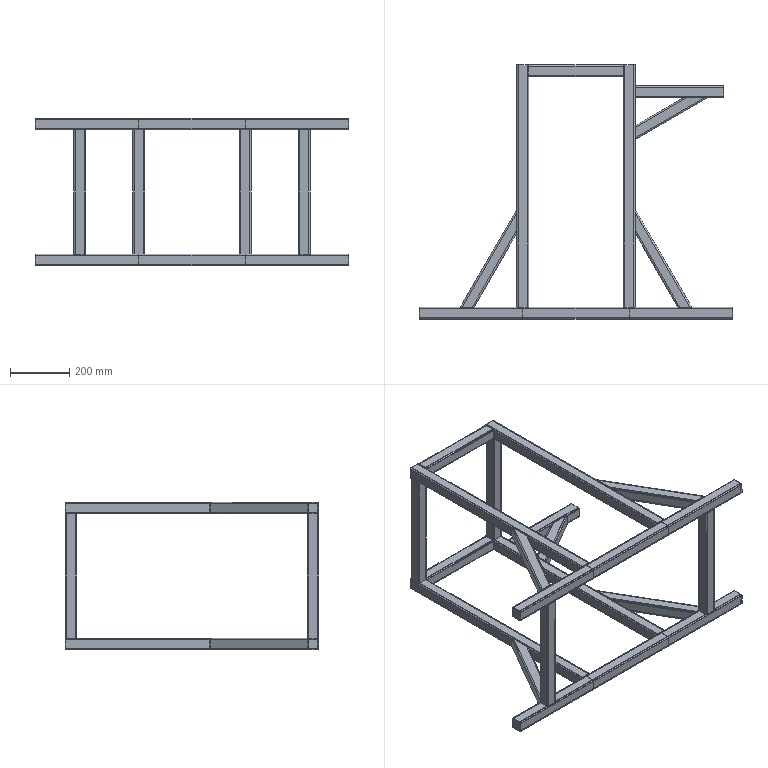Part | SolidWorks | features 3DProfileFeature 1, EndCap 1, WeldCornerFeat 1, WeldMemberFeat 1, WeldmentFeature 1 | 26 solids | 420 faces | box 1060 x 860 x 500 mm | volume 4110495 mm3 | plane 244 | cylinder 176 | commonest cylinder face diameters 4 x88 10 x88